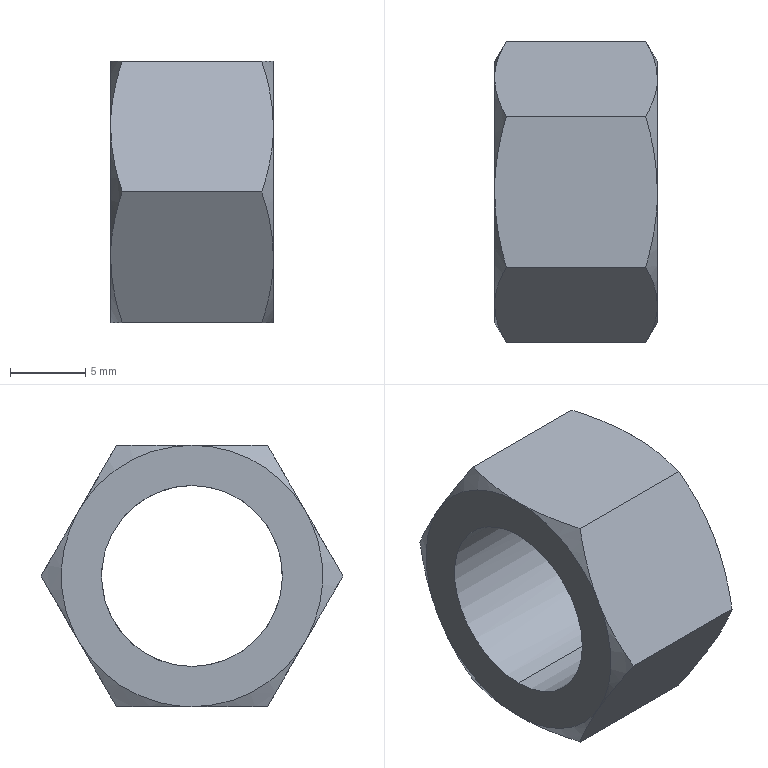Part | STEP file | Positioning_id1614_x_t | 1 solid | 22 faces | box 10.8 x 20.03 x 17.346 mm | volume 1581 mm3 | cone 12 | plane 8 | cylinder 2 | commonest cylinder face diameters 12 x2